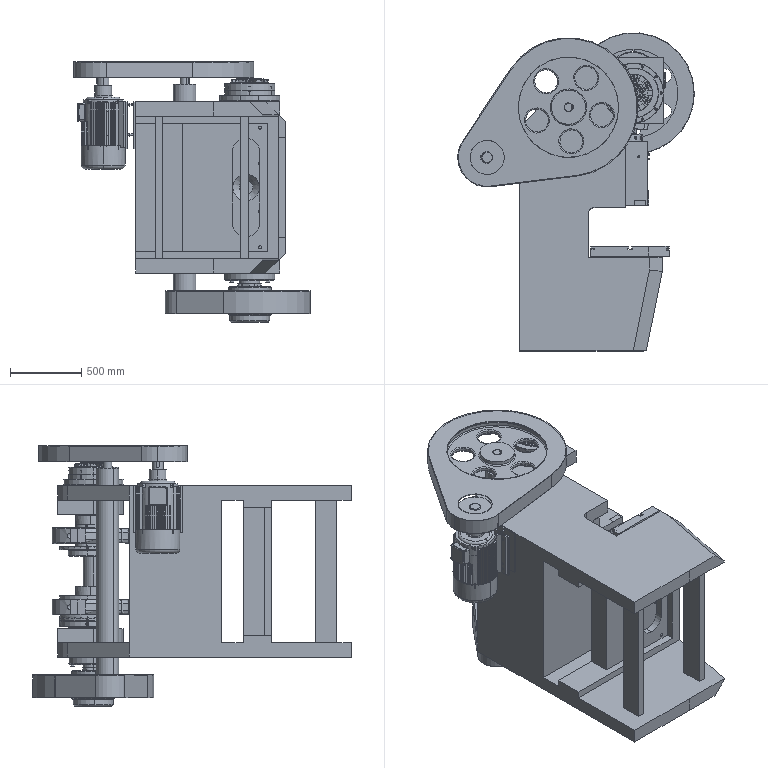Part | SolidWorks | 117 solids | 5986 faces | volume 951819714 mm3 | cylinder 2300 | plane 2068 | cone 572 | sphere 552 | torus 288 | spline 206 | commonest cylinder face diameters 3.8 x372 262.053 x157 262.284 x157 789.22 x156 12 x137 20 x102